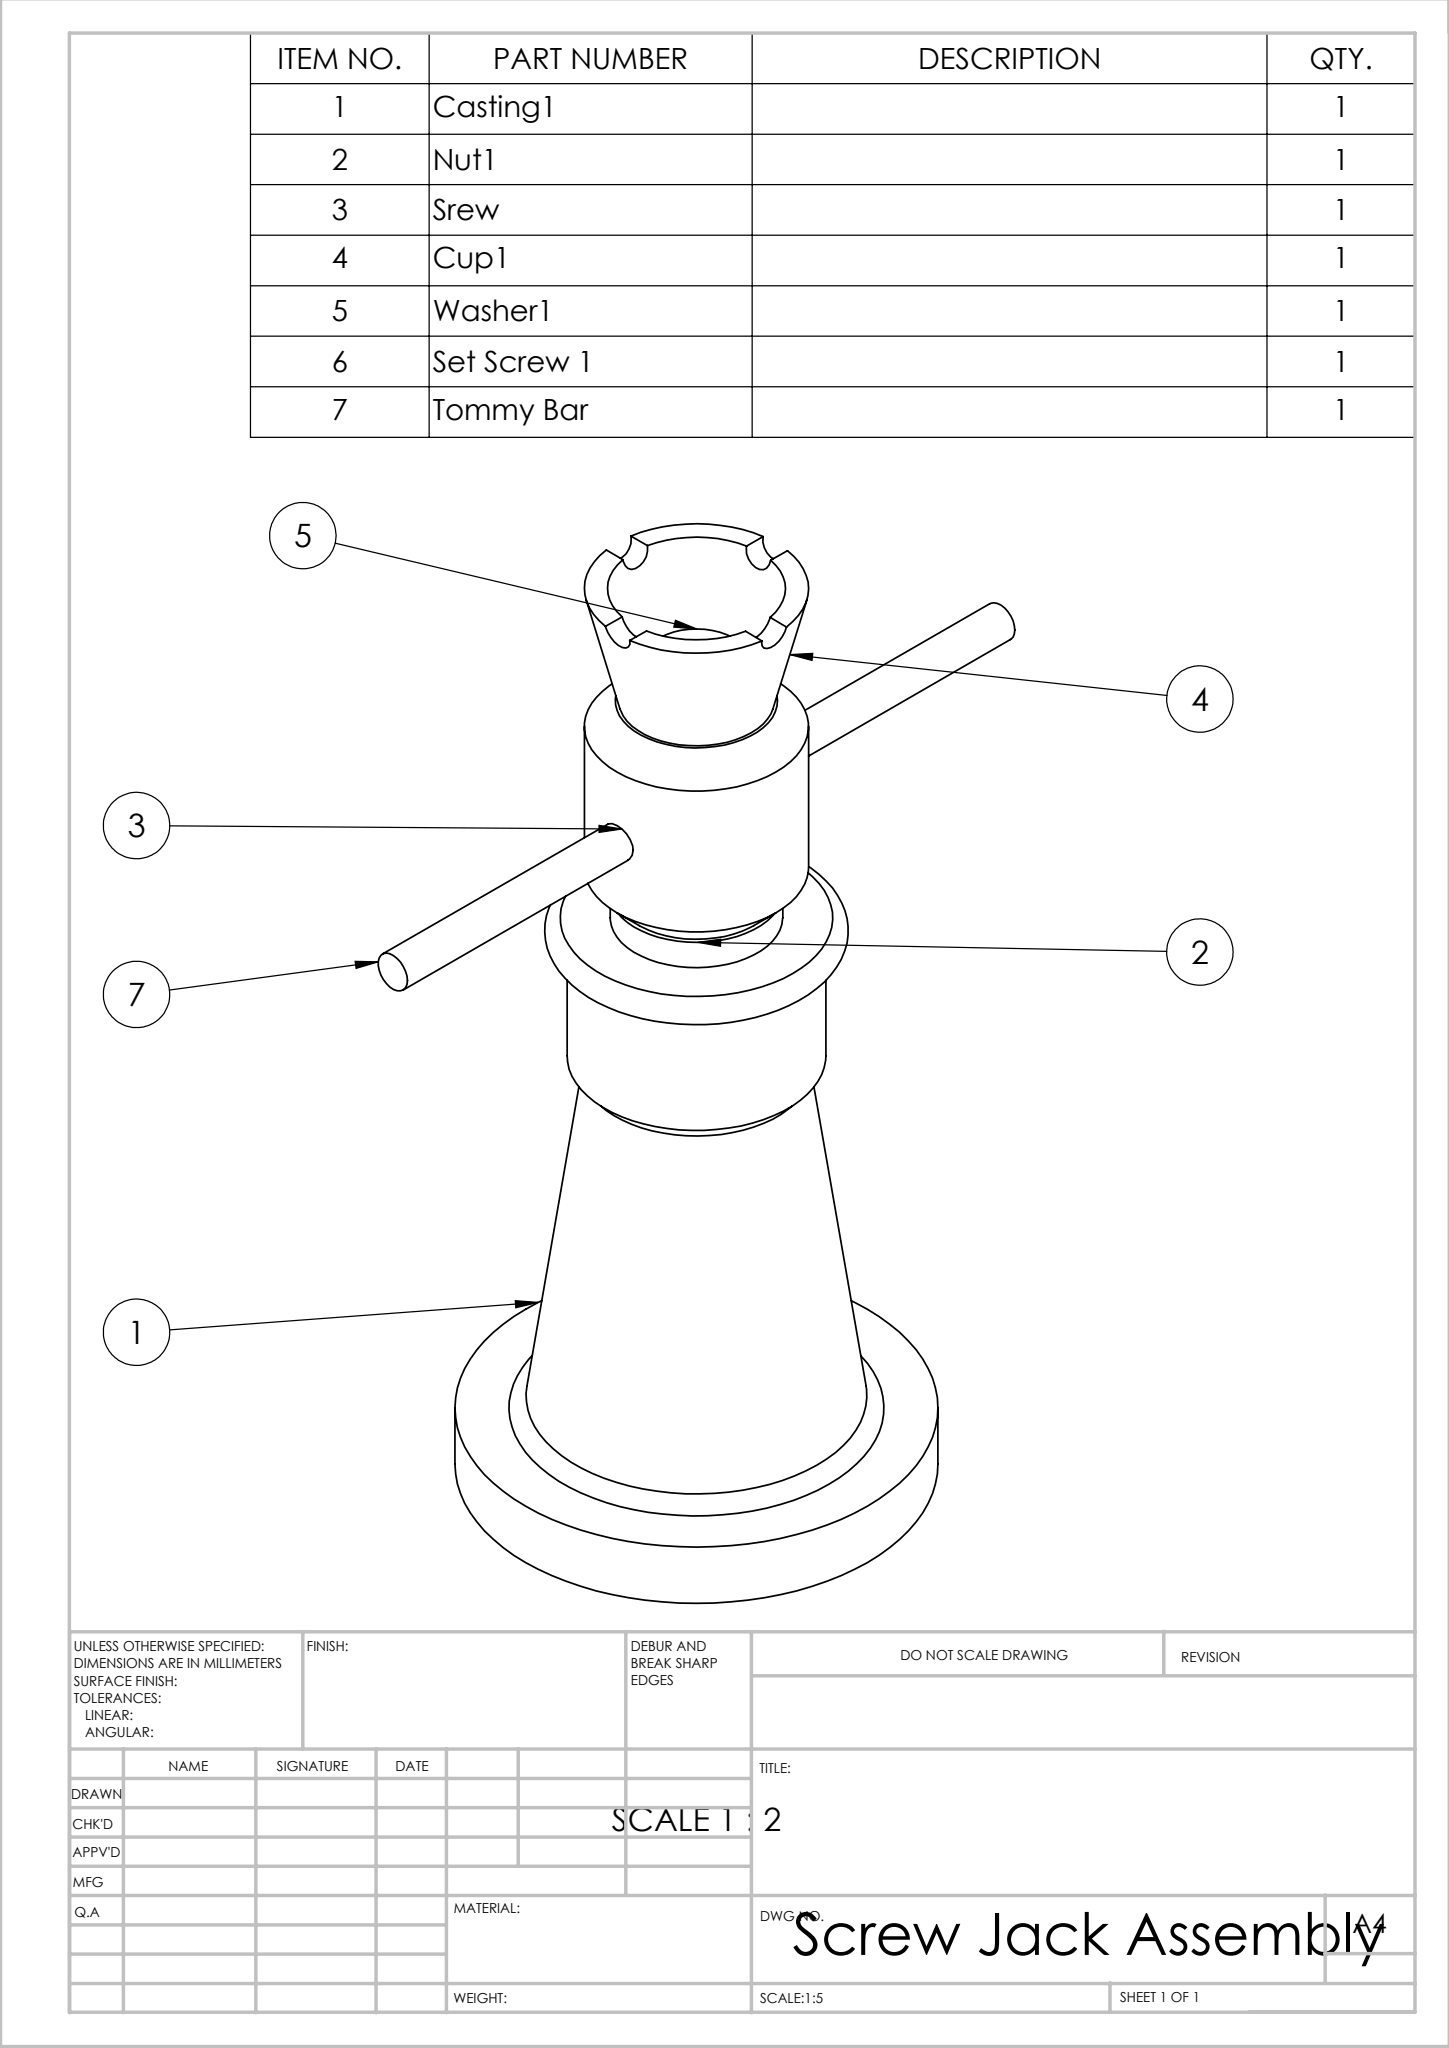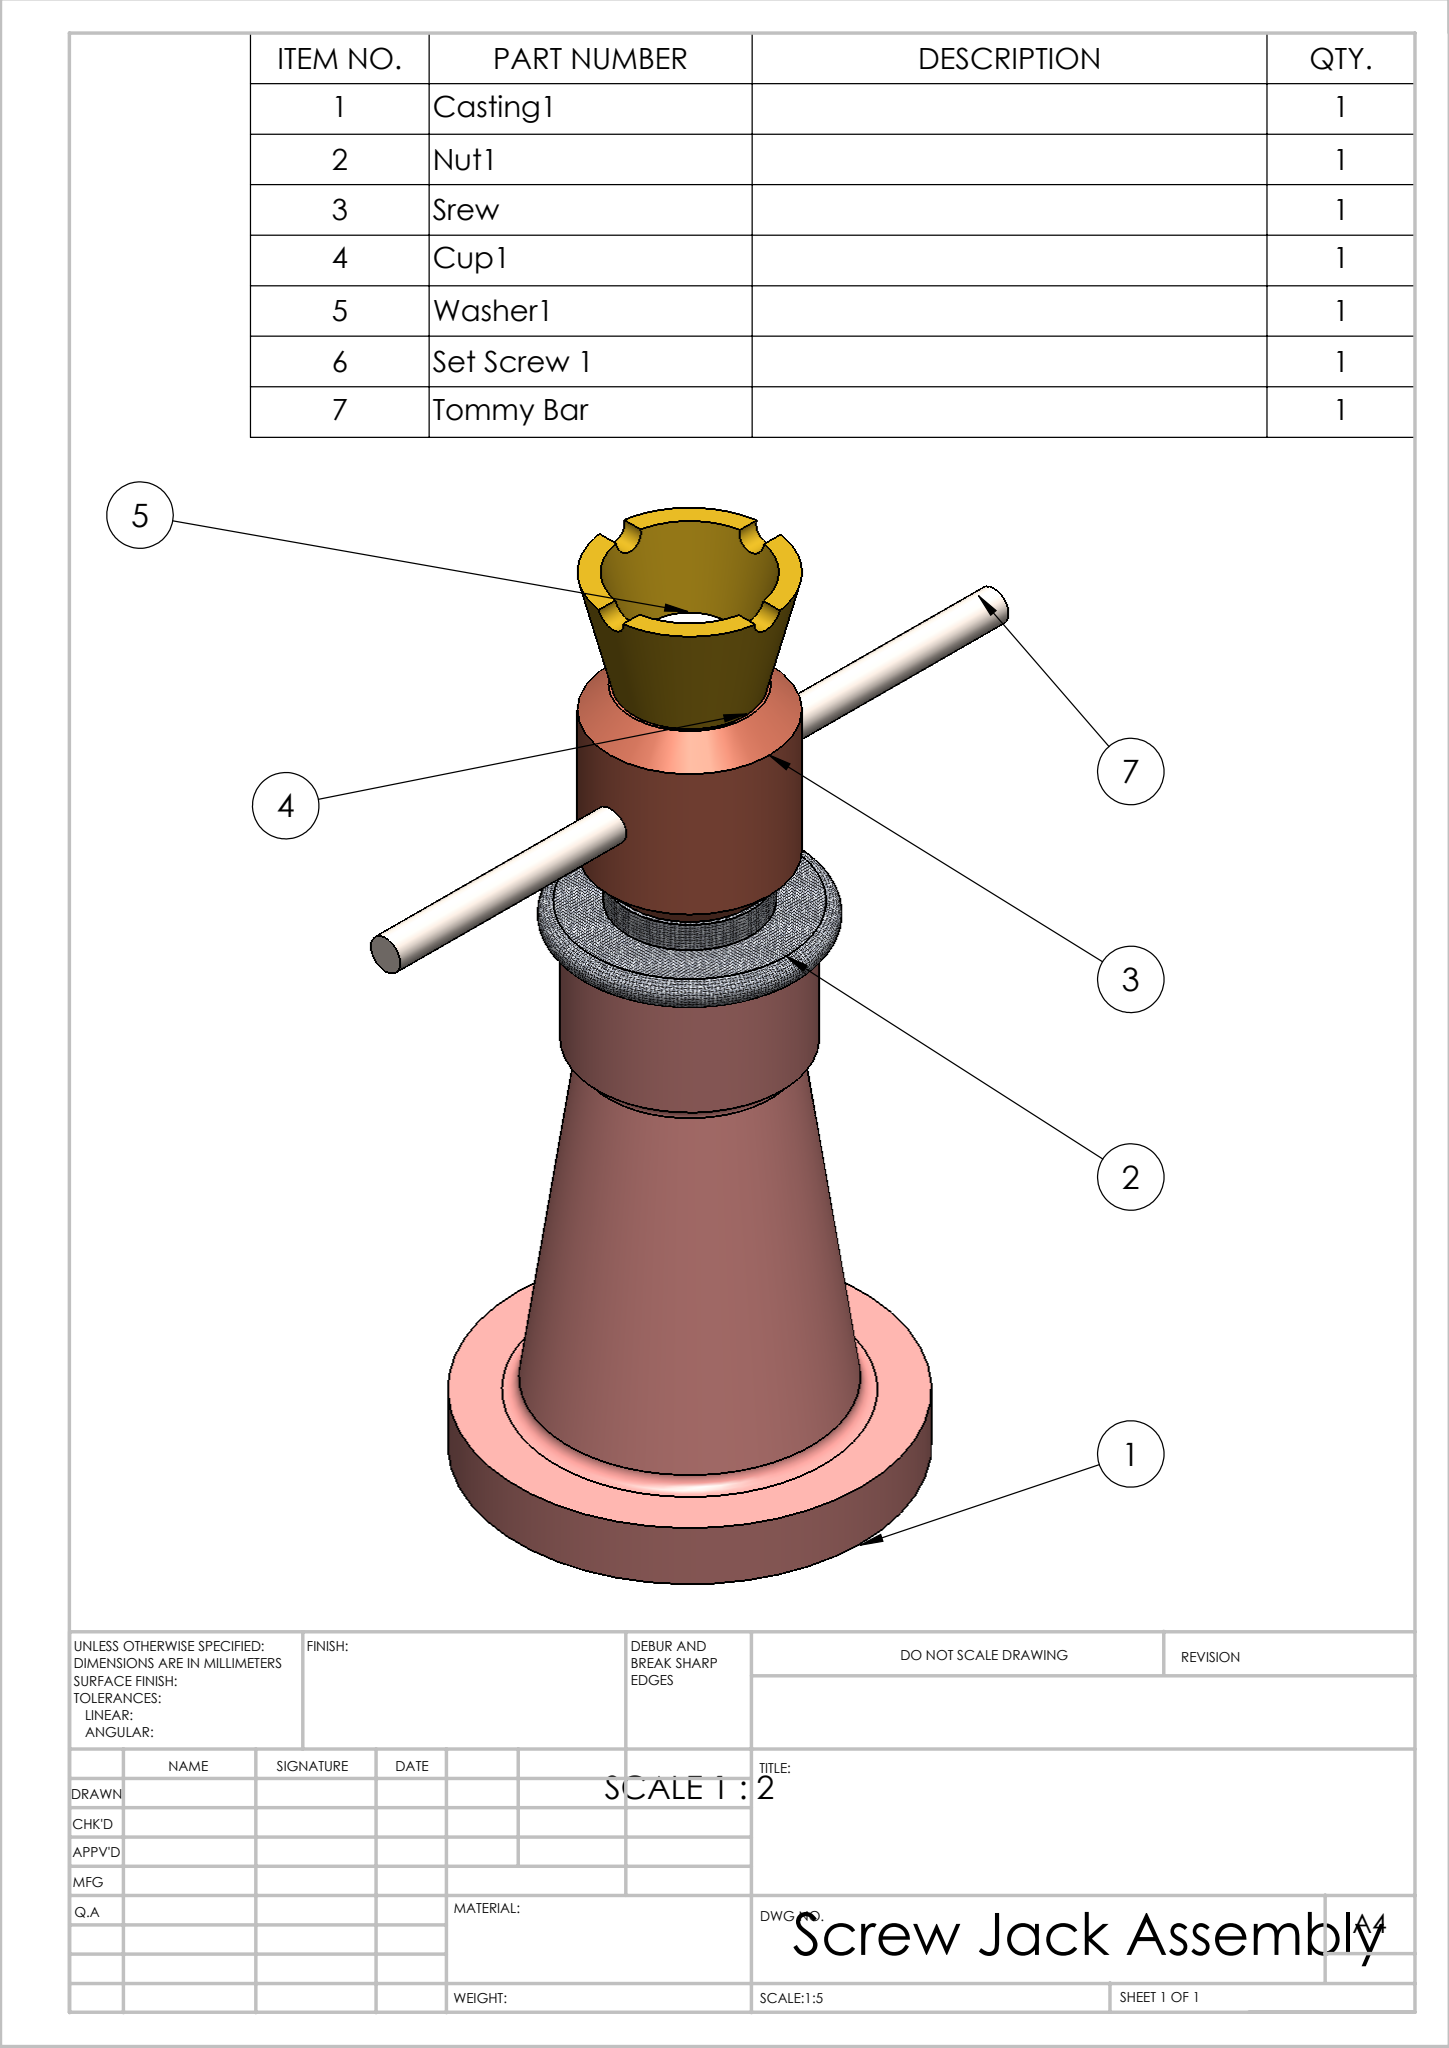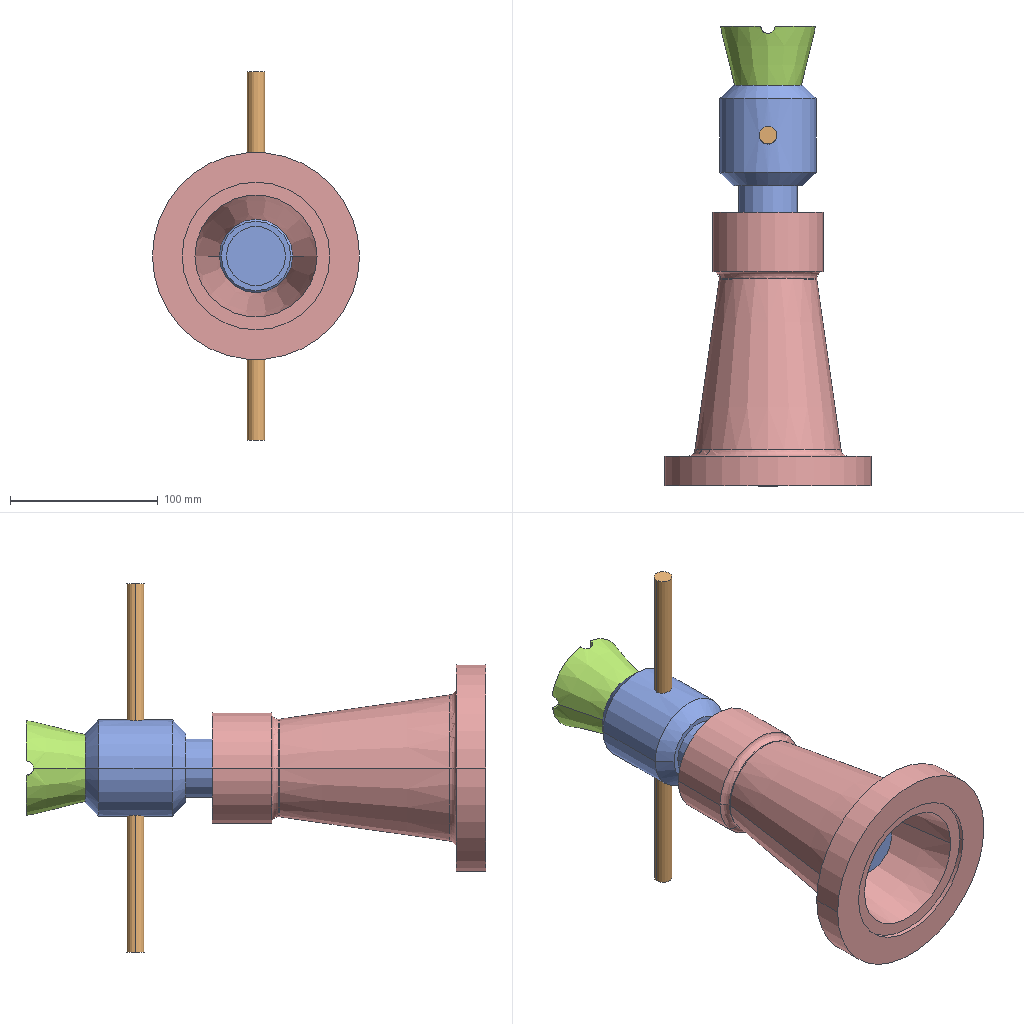Assembly | SolidWorks | 8 different items | 8 placed | box 140 x 311 x 249 mm
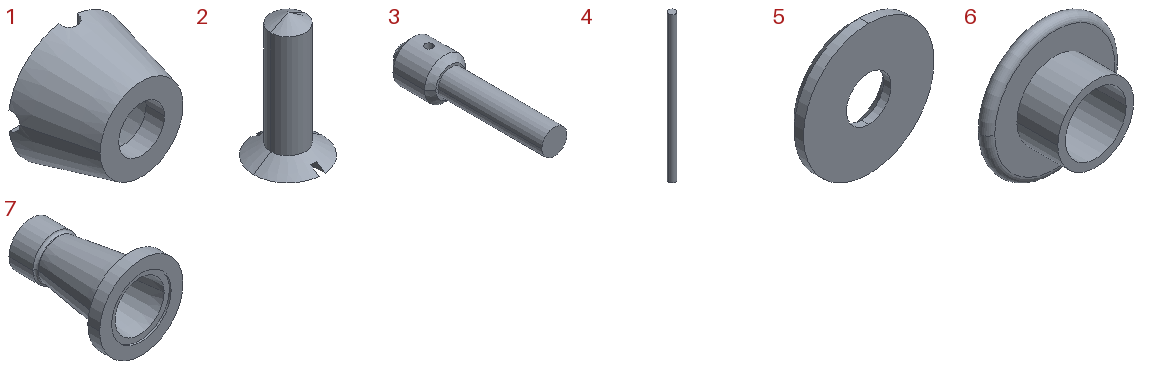Parts list (item | name | quantity | size | volume | features):
1 | - | x1 | 64.226 x 40 x 64.226 mm | 43850 mm3 | features ICE 2, CirPattern 1, Revolution 1
2 | - | x1 | 18 x 17.937 x 32.5 mm | 2181 mm3 | features ICE 1, Revolution 1
3 | - | x1 | 65 x 243 x 65 mm | 412398 mm3 | features ICE 1, RevCut 1, Revolution 1
4 | - | x1 | 12 x 12 x 249 mm | 28161 mm3 | features Extrusion 1
5 | - | x1 | 35 x 5 x 35 mm | 3720 mm3 | features Chamfer 1, Revolution 1
6 | - | x1 | 88 x 45 x 88 mm | 66528 mm3 | features Revolution 1
7 | - | x1 | 140 x 185 x 140 mm | 602194 mm3 | features Revolution 1
8 | Nut1 | x1 | - | - | -
Mates (type | each side: item.copy, entity, surface, feature):
Concentric | 3.1 face cylinder Cut-Revolve1 | 1.1 face cone Revolve1
Coincident | 3.1 face plane Revolve7 | 1.1 face plane Revolve1
Concentric | 3.1 face cylinder Cut-Revolve1 | 5.1 face cylinder Revolve1
Coincident | 1.1 face plane Revolve1 | 5.1 face plane Revolve1
Concentric | 5.1 face cylinder Revolve1 | 2.1 face cylinder Revolve3
Coincident | 5.1 face plane Revolve1 | 2.1 face plane Revolve3
Coincident | 3.1 plane | 4.1 plane
Concentric | 3.1 face cylinder Cut-Extrude1 | 4.1 face cylinder Boss-Extrude1